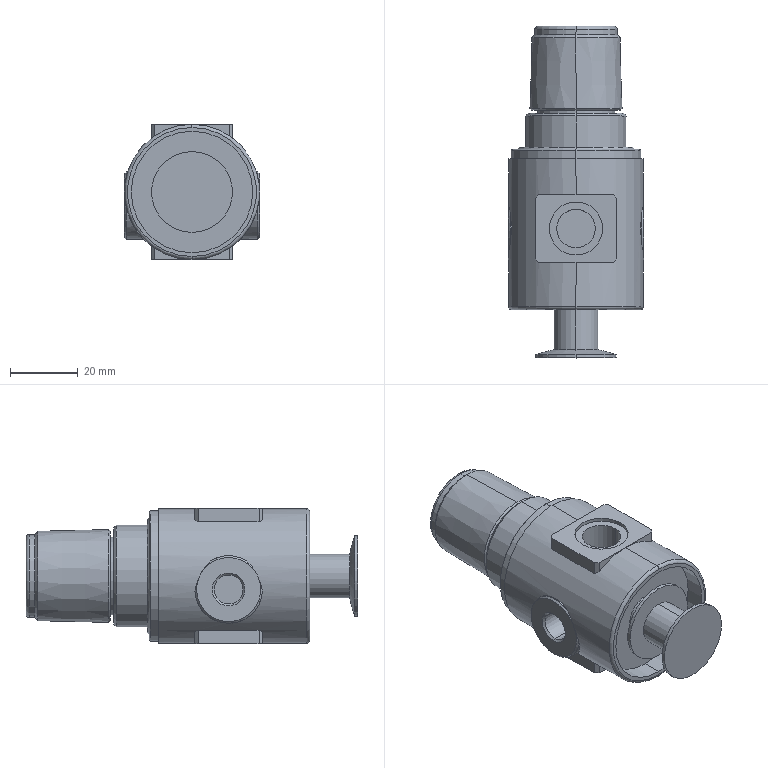Part | SolidWorks | features BaseBody 1 | 1 solid | 106 faces | box 40 x 98.3 x 40 mm | volume 76499 mm3 | plane 40 | cylinder 36 | cone 24 | torus 6 | commonest cylinder face diameters 8.566 x4 11.445 x4 13 x4 15.788 x4 20 x4 24 x4